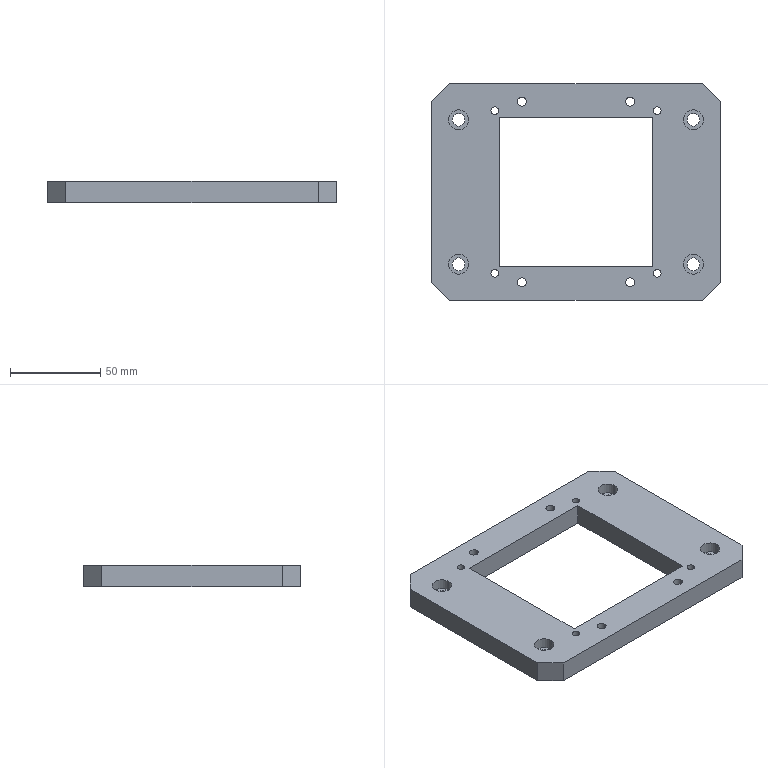Part | STEP file | magnetizing base plate | 1 solid | 50 faces | box 160 x 120 x 12 mm | volume 139548 mm3 | cylinder 32 | plane 18 | commonest cylinder face diameters 4.2 x8 5 x8 7 x8 11 x8